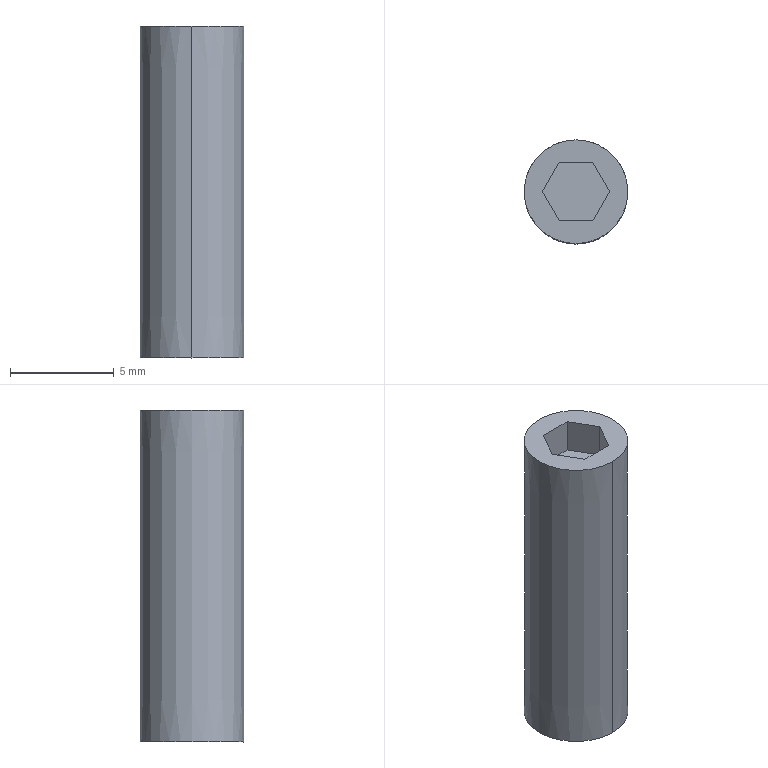Part | SolidWorks | features BaseBody 1 | 1 solid | 11 faces | box 5 x 5 x 16 mm | volume 302.585 mm3 | plane 9 | cone 2
STEP:
#1=CARTESIAN_POINT('',(571.645,-219.234,107.5));
#2=VERTEX_POINT('',#1);
#3=CARTESIAN_POINT('',(571.645,-214.236,107.5));
#4=VERTEX_POINT('',#3);
#5=CARTESIAN_POINT('',(571.645,-216.735,107.5));
#6=DIRECTION('',(0.,-0.000000003,1.));
#7=DIRECTION('',(0.,-1.,-0.000000003));
#8=AXIS2_PLACEMENT_3D('',#5,#6,#7);
#9=CIRCLE('',#8,2.499);
#10=EDGE_CURVE('',#2,#4,#9,.T.);
#11=ORIENTED_EDGE('',*,*,#10,.T.);
#12=CARTESIAN_POINT('',(571.645,-214.235,123.5));
#13=VERTEX_POINT('',#12);
#14=CARTESIAN_POINT('',(571.645,-214.235,123.5));
#15=DIRECTION('',(0.,0.00007812,1.));
#16=VECTOR('',#15,1000.);
#17=LINE('',#14,#16);
#18=EDGE_CURVE('',#4,#13,#17,.T.);
#19=ORIENTED_EDGE('',*,*,#18,.T.);
#20=CARTESIAN_POINT('',(571.645,-219.235,123.5));
#21=VERTEX_POINT('',#20);
#22=CARTESIAN_POINT('',(571.645,-216.735,123.5));
#23=DIRECTION('',(0.,0.000000003,-1.));
#24=DIRECTION('',(0.,-1.,-0.000000003));
#25=AXIS2_PLACEMENT_3D('',#22,#23,#24);
#26=CIRCLE('',#25,2.5);
#27=EDGE_CURVE('',#13,#21,#26,.T.);
#28=ORIENTED_EDGE('',*,*,#27,.T.);
#29=CARTESIAN_POINT('',(571.645,-219.235,123.5));
#30=DIRECTION('',(0.,-0.00007813,1.));
#31=VECTOR('',#30,1000.);
#32=LINE('',#29,#31);
#33=EDGE_CURVE('',#2,#21,#32,.T.);
#34=ORIENTED_EDGE('',*,*,#33,.F.);
#35=EDGE_LOOP('',(#11,#19,#28,#34));
#36=FACE_OUTER_BOUND('',#35,.T.);
#37=CARTESIAN_POINT('',(571.645,-216.735,123.5));
#38=DIRECTION('',(0.,-0.000000003,1.));
#39=DIRECTION('',(0.,-1.,-0.000000003));
#40=AXIS2_PLACEMENT_3D('',#37,#38,#39);
#41=CONICAL_SURFACE('',#40,2.5,0.00007812);
#42=ADVANCED_FACE('',(#36),#41,.T.);
#43=ORIENTED_EDGE('',*,*,#18,.F.);
#44=CARTESIAN_POINT('',(571.645,-216.735,107.5));
#45=DIRECTION('',(0.,-0.000000003,1.));
#46=DIRECTION('',(0.,-1.,-0.000000003));
#47=AXIS2_PLACEMENT_3D('',#44,#45,#46);
#48=CIRCLE('',#47,2.499);
#49=EDGE_CURVE('',#4,#2,#48,.T.);
#50=ORIENTED_EDGE('',*,*,#49,.T.);
#51=ORIENTED_EDGE('',*,*,#33,.T.);
#52=CARTESIAN_POINT('',(571.645,-216.735,123.5));
#53=DIRECTION('',(0.,0.000000003,-1.));
#54=DIRECTION('',(0.,-1.,-0.000000003));
#55=AXIS2_PLACEMENT_3D('',#52,#53,#54);
#56=CIRCLE('',#55,2.5);
#57=EDGE_CURVE('',#21,#13,#56,.T.);
#58=ORIENTED_EDGE('',*,*,#57,.T.);
#59=EDGE_LOOP('',(#43,#50,#51,#58));
#60=FACE_OUTER_BOUND('',#59,.T.);
#61=CARTESIAN_POINT('',(571.645,-216.735,123.5));
#62=DIRECTION('',(0.,-0.000000003,1.));
#63=DIRECTION('',(0.,-1.,-0.000000003));
#64=AXIS2_PLACEMENT_3D('',#61,#62,#63);
#65=CONICAL_SURFACE('',#64,2.5,0.00007812);
#66=ADVANCED_FACE('',(#60),#65,.T.);
#67=ORIENTED_EDGE('',*,*,#57,.F.);
#68=ORIENTED_EDGE('',*,*,#27,.F.);
#69=EDGE_LOOP('',(#67,#68));
#70=FACE_OUTER_BOUND('',#69,.T.);
#71=CARTESIAN_POINT('',(570.827,-215.332,123.5));
#72=VERTEX_POINT('',#71);
#73=CARTESIAN_POINT('',(572.451,-215.325,123.5));
#74=VERTEX_POINT('',#73);
#75=CARTESIAN_POINT('',(570.827,-215.332,123.5));
#76=DIRECTION('',(1.,0.004352,0.));
#77=VECTOR('',#76,1000.);
#78=LINE('',#75,#77);
#79=EDGE_CURVE('',#72,#74,#78,.T.);
#80=ORIENTED_EDGE('',*,*,#79,.T.);
#81=CARTESIAN_POINT('',(573.269,-216.728,123.5));
#82=VERTEX_POINT('',#81);
#83=CARTESIAN_POINT('',(572.451,-215.325,123.5));
#84=DIRECTION('',(0.5038,-0.8638,-0.000000003));
#85=VECTOR('',#84,1000.);
#86=LINE('',#83,#85);
#87=EDGE_CURVE('',#74,#82,#86,.T.);
#88=ORIENTED_EDGE('',*,*,#87,.T.);
#89=CARTESIAN_POINT('',(572.463,-218.138,123.5));
#90=VERTEX_POINT('',#89);
#91=CARTESIAN_POINT('',(573.269,-216.728,123.5));
#92=DIRECTION('',(-0.4962,-0.8682,-0.000000003));
#93=VECTOR('',#92,1000.);
#94=LINE('',#91,#93);
#95=EDGE_CURVE('',#82,#90,#94,.T.);
#96=ORIENTED_EDGE('',*,*,#95,.T.);
#97=CARTESIAN_POINT('',(570.839,-218.145,123.5));
#98=VERTEX_POINT('',#97);
#99=CARTESIAN_POINT('',(572.463,-218.138,123.5));
#100=DIRECTION('',(-1.,-0.004352,0.));
#101=VECTOR('',#100,1000.);
#102=LINE('',#99,#101);
#103=EDGE_CURVE('',#90,#98,#102,.T.);
#104=ORIENTED_EDGE('',*,*,#103,.T.);
#105=CARTESIAN_POINT('',(570.021,-216.742,123.5));
#106=VERTEX_POINT('',#105);
#107=CARTESIAN_POINT('',(570.839,-218.145,123.5));
#108=DIRECTION('',(-0.5038,0.8638,0.000000003));
#109=VECTOR('',#108,1000.);
#110=LINE('',#107,#109);
#111=EDGE_CURVE('',#98,#106,#110,.T.);
#112=ORIENTED_EDGE('',*,*,#111,.T.);
#113=CARTESIAN_POINT('',(570.021,-216.742,123.5));
#114=DIRECTION('',(0.4962,0.8682,0.000000003));
#115=VECTOR('',#114,1000.);
#116=LINE('',#113,#115);
#117=EDGE_CURVE('',#106,#72,#116,.T.);
#118=ORIENTED_EDGE('',*,*,#117,.T.);
#119=EDGE_LOOP('',(#80,#88,#96,#104,#112,#118));
#120=FACE_BOUND('',#119,.T.);
#121=CARTESIAN_POINT('',(571.651,-217.985,123.5));
#122=DIRECTION('',(0.,-0.000000003,1.));
#123=DIRECTION('',(0.,-1.,-0.000000003));
#124=AXIS2_PLACEMENT_3D('',#121,#122,#123);
#125=PLANE('',#124);
#126=ADVANCED_FACE('',(#70,#120),#125,.T.);
#127=ORIENTED_EDGE('',*,*,#10,.F.);
#128=ORIENTED_EDGE('',*,*,#49,.F.);
#129=EDGE_LOOP('',(#127,#128));
#130=FACE_OUTER_BOUND('',#129,.T.);
#131=CARTESIAN_POINT('',(571.651,-217.984,107.5));
#132=DIRECTION('',(0.,0.000000003,-1.));
#133=DIRECTION('',(0.,1.,0.000000003));
#134=AXIS2_PLACEMENT_3D('',#131,#132,#133);
#135=PLANE('',#134);
#136=ADVANCED_FACE('',(#130),#135,.T.);
#137=CARTESIAN_POINT('',(572.451,-215.325,121.833));
#138=VERTEX_POINT('',#137);
#139=CARTESIAN_POINT('',(572.451,-215.325,121.833));
#140=DIRECTION('',(-0.000000001,-0.000000001,1.));
#141=VECTOR('',#140,1000.);
#142=LINE('',#139,#141);
#143=EDGE_CURVE('',#138,#74,#142,.T.);
#144=ORIENTED_EDGE('',*,*,#143,.F.);
#145=CARTESIAN_POINT('',(573.269,-216.728,121.833));
#146=VERTEX_POINT('',#145);
#147=CARTESIAN_POINT('',(572.451,-215.325,121.833));
#148=DIRECTION('',(-0.5038,0.8638,0.));
#149=VECTOR('',#148,1000.);
#150=LINE('',#147,#149);
#151=EDGE_CURVE('',#146,#138,#150,.T.);
#152=ORIENTED_EDGE('',*,*,#151,.F.);
#153=CARTESIAN_POINT('',(573.269,-216.728,121.833));
#154=DIRECTION('',(0.000000001,0.000000001,-1.));
#155=VECTOR('',#154,1000.);
#156=LINE('',#153,#155);
#157=EDGE_CURVE('',#82,#146,#156,.T.);
#158=ORIENTED_EDGE('',*,*,#157,.F.);
#159=ORIENTED_EDGE('',*,*,#87,.F.);
#160=EDGE_LOOP('',(#144,#152,#158,#159));
#161=FACE_OUTER_BOUND('',#160,.T.);
#162=CARTESIAN_POINT('',(572.451,-215.325,121.833));
#163=DIRECTION('',(0.8638,0.5038,0.000000002));
#164=DIRECTION('',(-0.5038,0.8638,0.));
#165=AXIS2_PLACEMENT_3D('',#162,#163,#164);
#166=PLANE('',#165);
#167=ADVANCED_FACE('',(#161),#166,.F.);
#168=CARTESIAN_POINT('',(570.827,-215.332,121.833));
#169=VERTEX_POINT('',#168);
#170=CARTESIAN_POINT('',(570.827,-215.332,121.833));
#171=DIRECTION('',(0.,-0.000000003,1.));
#172=VECTOR('',#171,1000.);
#173=LINE('',#170,#172);
#174=EDGE_CURVE('',#169,#72,#173,.T.);
#175=ORIENTED_EDGE('',*,*,#174,.F.);
#176=CARTESIAN_POINT('',(570.827,-215.332,121.833));
#177=DIRECTION('',(-1.,-0.004352,0.));
#178=VECTOR('',#177,1000.);
#179=LINE('',#176,#178);
#180=EDGE_CURVE('',#138,#169,#179,.T.);
#181=ORIENTED_EDGE('',*,*,#180,.F.);
#182=ORIENTED_EDGE('',*,*,#143,.T.);
#183=ORIENTED_EDGE('',*,*,#79,.F.);
#184=EDGE_LOOP('',(#175,#181,#182,#183));
#185=FACE_OUTER_BOUND('',#184,.T.);
#186=CARTESIAN_POINT('',(570.827,-215.332,121.833));
#187=DIRECTION('',(-0.004352,1.,0.000000003));
#188=DIRECTION('',(-1.,-0.004352,0.));
#189=AXIS2_PLACEMENT_3D('',#186,#187,#188);
#190=PLANE('',#189);
#191=ADVANCED_FACE('',(#185),#190,.F.);
#192=CARTESIAN_POINT('',(570.021,-216.742,121.833));
#193=VERTEX_POINT('',#192);
#194=CARTESIAN_POINT('',(570.021,-216.742,121.833));
#195=DIRECTION('',(0.000000001,-0.000000001,1.));
#196=VECTOR('',#195,1000.);
#197=LINE('',#194,#196);
#198=EDGE_CURVE('',#193,#106,#197,.T.);
#199=ORIENTED_EDGE('',*,*,#198,.F.);
#200=CARTESIAN_POINT('',(570.021,-216.742,121.833));
#201=DIRECTION('',(-0.4962,-0.8682,0.));
#202=VECTOR('',#201,1000.);
#203=LINE('',#200,#202);
#204=EDGE_CURVE('',#169,#193,#203,.T.);
#205=ORIENTED_EDGE('',*,*,#204,.F.);
#206=ORIENTED_EDGE('',*,*,#174,.T.);
#207=ORIENTED_EDGE('',*,*,#117,.F.);
#208=EDGE_LOOP('',(#199,#205,#206,#207));
#209=FACE_OUTER_BOUND('',#208,.T.);
#210=CARTESIAN_POINT('',(570.021,-216.742,121.833));
#211=DIRECTION('',(-0.8682,0.4962,0.000000002));
#212=DIRECTION('',(-0.4962,-0.8682,0.));
#213=AXIS2_PLACEMENT_3D('',#210,#211,#212);
#214=PLANE('',#213);
#215=ADVANCED_FACE('',(#209),#214,.F.);
#216=CARTESIAN_POINT('',(570.839,-218.145,121.833));
#217=VERTEX_POINT('',#216);
#218=CARTESIAN_POINT('',(570.839,-218.145,121.833));
#219=DIRECTION('',(-0.000000001,-0.000000001,1.));
#220=VECTOR('',#219,1000.);
#221=LINE('',#218,#220);
#222=EDGE_CURVE('',#217,#98,#221,.T.);
#223=ORIENTED_EDGE('',*,*,#222,.F.);
#224=CARTESIAN_POINT('',(570.839,-218.145,121.833));
#225=DIRECTION('',(0.5038,-0.8638,0.));
#226=VECTOR('',#225,1000.);
#227=LINE('',#224,#226);
#228=EDGE_CURVE('',#193,#217,#227,.T.);
#229=ORIENTED_EDGE('',*,*,#228,.F.);
#230=ORIENTED_EDGE('',*,*,#198,.T.);
#231=ORIENTED_EDGE('',*,*,#111,.F.);
#232=EDGE_LOOP('',(#223,#229,#230,#231));
#233=FACE_OUTER_BOUND('',#232,.T.);
#234=CARTESIAN_POINT('',(570.839,-218.145,121.833));
#235=DIRECTION('',(-0.8638,-0.5038,-0.000000002));
#236=DIRECTION('',(0.5038,-0.8638,0.));
#237=AXIS2_PLACEMENT_3D('',#234,#235,#236);
#238=PLANE('',#237);
#239=ADVANCED_FACE('',(#233),#238,.F.);
#240=CARTESIAN_POINT('',(572.463,-218.138,121.833));
#241=VERTEX_POINT('',#240);
#242=CARTESIAN_POINT('',(572.463,-218.138,121.833));
#243=DIRECTION('',(0.,-0.000000003,1.));
#244=VECTOR('',#243,1000.);
#245=LINE('',#242,#244);
#246=EDGE_CURVE('',#241,#90,#245,.T.);
#247=ORIENTED_EDGE('',*,*,#246,.F.);
#248=CARTESIAN_POINT('',(572.463,-218.138,121.833));
#249=DIRECTION('',(1.,0.004352,0.));
#250=VECTOR('',#249,1000.);
#251=LINE('',#248,#250);
#252=EDGE_CURVE('',#217,#241,#251,.T.);
#253=ORIENTED_EDGE('',*,*,#252,.F.);
#254=ORIENTED_EDGE('',*,*,#222,.T.);
#255=ORIENTED_EDGE('',*,*,#103,.F.);
#256=EDGE_LOOP('',(#247,#253,#254,#255));
#257=FACE_OUTER_BOUND('',#256,.T.);
#258=CARTESIAN_POINT('',(572.463,-218.138,121.833));
#259=DIRECTION('',(0.004352,-1.,-0.000000003));
#260=DIRECTION('',(1.,0.004352,0.));
#261=AXIS2_PLACEMENT_3D('',#258,#259,#260);
#262=PLANE('',#261);
#263=ADVANCED_FACE('',(#257),#262,.F.);
#264=ORIENTED_EDGE('',*,*,#157,.T.);
#265=CARTESIAN_POINT('',(573.269,-216.728,121.833));
#266=DIRECTION('',(0.4962,0.8682,0.));
#267=VECTOR('',#266,1000.);
#268=LINE('',#265,#267);
#269=EDGE_CURVE('',#241,#146,#268,.T.);
#270=ORIENTED_EDGE('',*,*,#269,.F.);
#271=ORIENTED_EDGE('',*,*,#246,.T.);
#272=ORIENTED_EDGE('',*,*,#95,.F.);
#273=EDGE_LOOP('',(#264,#270,#271,#272));
#274=FACE_OUTER_BOUND('',#273,.T.);
#275=CARTESIAN_POINT('',(573.269,-216.728,121.833));
#276=DIRECTION('',(0.8682,-0.4962,-0.000000002));
#277=DIRECTION('',(0.4962,0.8682,0.));
#278=AXIS2_PLACEMENT_3D('',#275,#276,#277);
#279=PLANE('',#278);
#280=ADVANCED_FACE('',(#274),#279,.F.);
#281=ORIENTED_EDGE('',*,*,#252,.T.);
#282=ORIENTED_EDGE('',*,*,#269,.T.);
#283=ORIENTED_EDGE('',*,*,#151,.T.);
#284=ORIENTED_EDGE('',*,*,#180,.T.);
#285=ORIENTED_EDGE('',*,*,#204,.T.);
#286=ORIENTED_EDGE('',*,*,#228,.T.);
#287=EDGE_LOOP('',(#281,#282,#283,#284,#285,#286));
#288=FACE_OUTER_BOUND('',#287,.T.);
#289=CARTESIAN_POINT('',(571.645,-216.735,121.833));
#290=DIRECTION('',(0.,-0.000000003,1.));
#291=DIRECTION('',(0.,-1.,-0.000000003));
#292=AXIS2_PLACEMENT_3D('',#289,#290,#291);
#293=PLANE('',#292);
#294=ADVANCED_FACE('',(#288),#293,.T.);
#295=CLOSED_SHELL('',(#42,#66,#126,#136,#167,#191,#215,#239,#263,#280,#294));
#296=MANIFOLD_SOLID_BREP('',#295);
#297=CARTESIAN_POINT('',(0.,0.,0.));
#298=DIRECTION('',(0.,0.,1.));
#299=DIRECTION('',(1.,0.,0.));
#300=AXIS2_PLACEMENT_3D('',#297,#298,#299);
#301=(LENGTH_UNIT()NAMED_UNIT(*)SI_UNIT(.MILLI.,.METRE.));
#302=UNCERTAINTY_MEASURE_WITH_UNIT(LENGTH_MEASURE(0.00001),#301,'','');
#303=(NAMED_UNIT(*)PLANE_ANGLE_UNIT()SI_UNIT($,.RADIAN.));
#304=(NAMED_UNIT(*)SI_UNIT($,.STERADIAN.)SOLID_ANGLE_UNIT());
#305=(GEOMETRIC_REPRESENTATION_CONTEXT(3)GLOBAL_UNCERTAINTY_ASSIGNED_CONTEXT((#302))GLOBAL_UNIT_ASSIGNED_CONTEXT((#301,#303,#304))REPRESENTATION_CONTEXT('',''));
#306=ADVANCED_BREP_SHAPE_REPRESENTATION('',(#296,#300),#305);